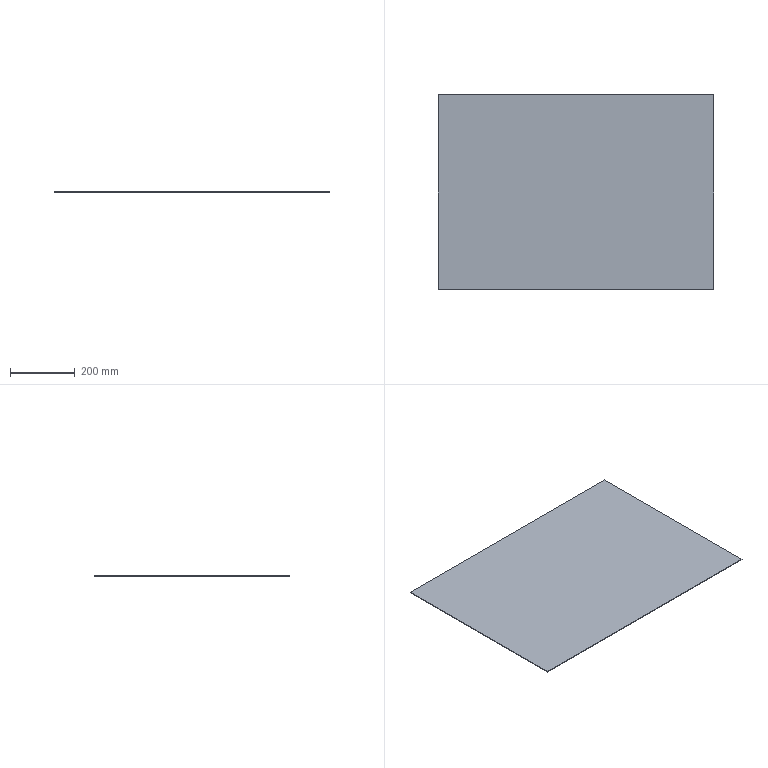Part | SolidWorks | features FlatPattern 1, SMBaseFlange 1, SheetMetal 1 | 1 solid | 6 faces | box 850 x 600 x 2 mm | volume 1020000 mm3 | plane 6
STEP:
#1=CARTESIAN_POINT('',(425.,-300.,0.));
#2=VERTEX_POINT('',#1);
#3=CARTESIAN_POINT('',(425.,300.,0.));
#4=VERTEX_POINT('',#3);
#5=CARTESIAN_POINT('',(425.,-300.,0.));
#6=DIRECTION('',(0.,1.,0.));
#7=VECTOR('',#6,1000.);
#8=LINE('',#5,#7);
#9=EDGE_CURVE('',#2,#4,#8,.T.);
#10=ORIENTED_EDGE('',*,*,#9,.F.);
#11=CARTESIAN_POINT('',(425.,-300.,-2.));
#12=VERTEX_POINT('',#11);
#13=CARTESIAN_POINT('',(425.,-300.,-2.));
#14=DIRECTION('',(0.,0.,1.));
#15=VECTOR('',#14,1000.);
#16=LINE('',#13,#15);
#17=EDGE_CURVE('',#12,#2,#16,.T.);
#18=ORIENTED_EDGE('',*,*,#17,.F.);
#19=CARTESIAN_POINT('',(425.,300.,-2.));
#20=VERTEX_POINT('',#19);
#21=CARTESIAN_POINT('',(425.,-300.,-2.));
#22=DIRECTION('',(0.,1.,0.));
#23=VECTOR('',#22,1000.);
#24=LINE('',#21,#23);
#25=EDGE_CURVE('',#12,#20,#24,.T.);
#26=ORIENTED_EDGE('',*,*,#25,.T.);
#27=CARTESIAN_POINT('',(425.,300.,-2.));
#28=DIRECTION('',(0.,0.,1.));
#29=VECTOR('',#28,1000.);
#30=LINE('',#27,#29);
#31=EDGE_CURVE('',#20,#4,#30,.T.);
#32=ORIENTED_EDGE('',*,*,#31,.T.);
#33=EDGE_LOOP('',(#10,#18,#26,#32));
#34=FACE_OUTER_BOUND('',#33,.T.);
#35=CARTESIAN_POINT('',(425.,-300.,-2.));
#36=DIRECTION('',(1.,0.,0.));
#37=DIRECTION('',(0.,0.,-1.));
#38=AXIS2_PLACEMENT_3D('',#35,#36,#37);
#39=PLANE('',#38);
#40=ADVANCED_FACE('',(#34),#39,.T.);
#41=CARTESIAN_POINT('',(-425.,-300.,0.));
#42=VERTEX_POINT('',#41);
#43=CARTESIAN_POINT('',(-425.,-300.,0.));
#44=DIRECTION('',(1.,0.,0.));
#45=VECTOR('',#44,1000.);
#46=LINE('',#43,#45);
#47=EDGE_CURVE('',#42,#2,#46,.T.);
#48=ORIENTED_EDGE('',*,*,#47,.F.);
#49=CARTESIAN_POINT('',(-425.,-300.,-2.));
#50=VERTEX_POINT('',#49);
#51=CARTESIAN_POINT('',(-425.,-300.,-2.));
#52=DIRECTION('',(0.,0.,1.));
#53=VECTOR('',#52,1000.);
#54=LINE('',#51,#53);
#55=EDGE_CURVE('',#50,#42,#54,.T.);
#56=ORIENTED_EDGE('',*,*,#55,.F.);
#57=CARTESIAN_POINT('',(-425.,-300.,-2.));
#58=DIRECTION('',(1.,0.,0.));
#59=VECTOR('',#58,1000.);
#60=LINE('',#57,#59);
#61=EDGE_CURVE('',#50,#12,#60,.T.);
#62=ORIENTED_EDGE('',*,*,#61,.T.);
#63=ORIENTED_EDGE('',*,*,#17,.T.);
#64=EDGE_LOOP('',(#48,#56,#62,#63));
#65=FACE_OUTER_BOUND('',#64,.T.);
#66=CARTESIAN_POINT('',(-425.,-300.,-2.));
#67=DIRECTION('',(0.,-1.,0.));
#68=DIRECTION('',(0.,0.,-1.));
#69=AXIS2_PLACEMENT_3D('',#66,#67,#68);
#70=PLANE('',#69);
#71=ADVANCED_FACE('',(#65),#70,.T.);
#72=CARTESIAN_POINT('',(-425.,300.,0.));
#73=VERTEX_POINT('',#72);
#74=CARTESIAN_POINT('',(-425.,-300.,0.));
#75=DIRECTION('',(0.,-1.,0.));
#76=VECTOR('',#75,1000.);
#77=LINE('',#74,#76);
#78=EDGE_CURVE('',#73,#42,#77,.T.);
#79=ORIENTED_EDGE('',*,*,#78,.F.);
#80=CARTESIAN_POINT('',(-425.,300.,-2.));
#81=VERTEX_POINT('',#80);
#82=CARTESIAN_POINT('',(-425.,300.,-2.));
#83=DIRECTION('',(0.,0.,1.));
#84=VECTOR('',#83,1000.);
#85=LINE('',#82,#84);
#86=EDGE_CURVE('',#81,#73,#85,.T.);
#87=ORIENTED_EDGE('',*,*,#86,.F.);
#88=CARTESIAN_POINT('',(-425.,-300.,-2.));
#89=DIRECTION('',(0.,-1.,0.));
#90=VECTOR('',#89,1000.);
#91=LINE('',#88,#90);
#92=EDGE_CURVE('',#81,#50,#91,.T.);
#93=ORIENTED_EDGE('',*,*,#92,.T.);
#94=ORIENTED_EDGE('',*,*,#55,.T.);
#95=EDGE_LOOP('',(#79,#87,#93,#94));
#96=FACE_OUTER_BOUND('',#95,.T.);
#97=CARTESIAN_POINT('',(-425.,-300.,-2.));
#98=DIRECTION('',(-1.,0.,0.));
#99=DIRECTION('',(0.,0.,1.));
#100=AXIS2_PLACEMENT_3D('',#97,#98,#99);
#101=PLANE('',#100);
#102=ADVANCED_FACE('',(#96),#101,.T.);
#103=CARTESIAN_POINT('',(-425.,300.,0.));
#104=DIRECTION('',(-1.,0.,0.));
#105=VECTOR('',#104,1000.);
#106=LINE('',#103,#105);
#107=EDGE_CURVE('',#4,#73,#106,.T.);
#108=ORIENTED_EDGE('',*,*,#107,.F.);
#109=ORIENTED_EDGE('',*,*,#31,.F.);
#110=CARTESIAN_POINT('',(-425.,300.,-2.));
#111=DIRECTION('',(-1.,0.,0.));
#112=VECTOR('',#111,1000.);
#113=LINE('',#110,#112);
#114=EDGE_CURVE('',#20,#81,#113,.T.);
#115=ORIENTED_EDGE('',*,*,#114,.T.);
#116=ORIENTED_EDGE('',*,*,#86,.T.);
#117=EDGE_LOOP('',(#108,#109,#115,#116));
#118=FACE_OUTER_BOUND('',#117,.T.);
#119=CARTESIAN_POINT('',(-425.,300.,-2.));
#120=DIRECTION('',(0.,1.,0.));
#121=DIRECTION('',(0.,0.,1.));
#122=AXIS2_PLACEMENT_3D('',#119,#120,#121);
#123=PLANE('',#122);
#124=ADVANCED_FACE('',(#118),#123,.T.);
#125=ORIENTED_EDGE('',*,*,#25,.F.);
#126=ORIENTED_EDGE('',*,*,#61,.F.);
#127=ORIENTED_EDGE('',*,*,#92,.F.);
#128=ORIENTED_EDGE('',*,*,#114,.F.);
#129=EDGE_LOOP('',(#125,#126,#127,#128));
#130=FACE_OUTER_BOUND('',#129,.T.);
#131=CARTESIAN_POINT('',(0.,0.,-2.));
#132=DIRECTION('',(0.,0.,-1.));
#133=DIRECTION('',(-1.,0.,0.));
#134=AXIS2_PLACEMENT_3D('',#131,#132,#133);
#135=PLANE('',#134);
#136=ADVANCED_FACE('',(#130),#135,.T.);
#137=ORIENTED_EDGE('',*,*,#9,.T.);
#138=ORIENTED_EDGE('',*,*,#107,.T.);
#139=ORIENTED_EDGE('',*,*,#78,.T.);
#140=ORIENTED_EDGE('',*,*,#47,.T.);
#141=EDGE_LOOP('',(#137,#138,#139,#140));
#142=FACE_OUTER_BOUND('',#141,.T.);
#143=CARTESIAN_POINT('',(0.,0.,0.));
#144=DIRECTION('',(0.,0.,-1.));
#145=DIRECTION('',(-1.,0.,0.));
#146=AXIS2_PLACEMENT_3D('',#143,#144,#145);
#147=PLANE('',#146);
#148=ADVANCED_FACE('',(#142),#147,.F.);
#149=CLOSED_SHELL('',(#40,#71,#102,#124,#136,#148));
#150=MANIFOLD_SOLID_BREP('',#149);
#151=CARTESIAN_POINT('',(0.,0.,0.));
#152=DIRECTION('',(0.,0.,1.));
#153=DIRECTION('',(1.,0.,0.));
#154=AXIS2_PLACEMENT_3D('',#151,#152,#153);
#155=(LENGTH_UNIT()NAMED_UNIT(*)SI_UNIT(.MILLI.,.METRE.));
#156=UNCERTAINTY_MEASURE_WITH_UNIT(LENGTH_MEASURE(0.00001),#155,'','');
#157=(NAMED_UNIT(*)PLANE_ANGLE_UNIT()SI_UNIT($,.RADIAN.));
#158=(NAMED_UNIT(*)SI_UNIT($,.STERADIAN.)SOLID_ANGLE_UNIT());
#159=(GEOMETRIC_REPRESENTATION_CONTEXT(3)GLOBAL_UNCERTAINTY_ASSIGNED_CONTEXT((#156))GLOBAL_UNIT_ASSIGNED_CONTEXT((#155,#157,#158))REPRESENTATION_CONTEXT('',''));
#160=ADVANCED_BREP_SHAPE_REPRESENTATION('',(#150,#154),#159);